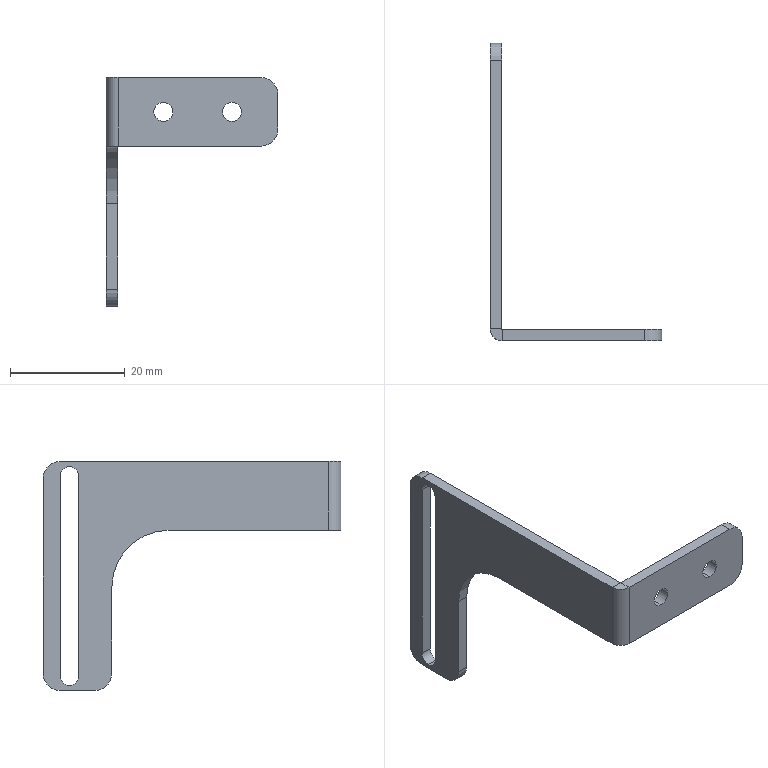Part | SolidWorks | features Fillet 2, ICE 2, FlatPattern 1, HoleWzd 1, SMBaseFlange 1, SheetMetal 1 | 1 solid | 29 faces | box 30 x 52 x 40 mm | volume 2330 mm3 | cylinder 15 | plane 14 | commonest cylinder face diameters 6 x5 3.3 x4 3.2 x3 0.2 x1 4.2 x1 20 x1
STEP:
#1=CARTESIAN_POINT('',(8.,-2.,32.35));
#2=VERTEX_POINT('',#1);
#3=CARTESIAN_POINT('',(8.,-2.,35.65));
#4=VERTEX_POINT('',#3);
#5=CARTESIAN_POINT('',(8.,-2.,34.));
#6=DIRECTION('',(0.,1.,0.));
#7=DIRECTION('',(0.,0.,1.));
#8=AXIS2_PLACEMENT_3D('',#5,#6,#7);
#9=CIRCLE('',#8,1.65);
#10=EDGE_CURVE('',#2,#4,#9,.T.);
#11=ORIENTED_EDGE('',*,*,#10,.F.);
#12=CARTESIAN_POINT('',(8.,0.,32.35));
#13=VERTEX_POINT('',#12);
#14=CARTESIAN_POINT('',(8.,0.,32.35));
#15=DIRECTION('',(0.,1.,0.));
#16=VECTOR('',#15,1000.);
#17=LINE('',#14,#16);
#18=EDGE_CURVE('',#2,#13,#17,.T.);
#19=ORIENTED_EDGE('',*,*,#18,.T.);
#20=CARTESIAN_POINT('',(8.,0.,35.65));
#21=VERTEX_POINT('',#20);
#22=CARTESIAN_POINT('',(8.,0.,34.));
#23=DIRECTION('',(0.,1.,0.));
#24=DIRECTION('',(0.,0.,1.));
#25=AXIS2_PLACEMENT_3D('',#22,#23,#24);
#26=CIRCLE('',#25,1.65);
#27=EDGE_CURVE('',#13,#21,#26,.T.);
#28=ORIENTED_EDGE('',*,*,#27,.T.);
#29=CARTESIAN_POINT('',(8.,0.,35.65));
#30=DIRECTION('',(0.,1.,0.));
#31=VECTOR('',#30,1000.);
#32=LINE('',#29,#31);
#33=EDGE_CURVE('',#4,#21,#32,.T.);
#34=ORIENTED_EDGE('',*,*,#33,.F.);
#35=EDGE_LOOP('',(#11,#19,#28,#34));
#36=FACE_OUTER_BOUND('',#35,.T.);
#37=CARTESIAN_POINT('',(8.,0.,34.));
#38=DIRECTION('',(0.,1.,0.));
#39=DIRECTION('',(0.,0.,1.));
#40=AXIS2_PLACEMENT_3D('',#37,#38,#39);
#41=CYLINDRICAL_SURFACE('',#40,1.65);
#42=ADVANCED_FACE('',(#36),#41,.F.);
#43=CARTESIAN_POINT('',(20.,-2.,32.35));
#44=VERTEX_POINT('',#43);
#45=CARTESIAN_POINT('',(20.,-2.,35.65));
#46=VERTEX_POINT('',#45);
#47=CARTESIAN_POINT('',(20.,-2.,34.));
#48=DIRECTION('',(0.,1.,0.));
#49=DIRECTION('',(0.,0.,1.));
#50=AXIS2_PLACEMENT_3D('',#47,#48,#49);
#51=CIRCLE('',#50,1.65);
#52=EDGE_CURVE('',#44,#46,#51,.T.);
#53=ORIENTED_EDGE('',*,*,#52,.F.);
#54=CARTESIAN_POINT('',(20.,0.,32.35));
#55=VERTEX_POINT('',#54);
#56=CARTESIAN_POINT('',(20.,0.,32.35));
#57=DIRECTION('',(0.,1.,0.));
#58=VECTOR('',#57,1000.);
#59=LINE('',#56,#58);
#60=EDGE_CURVE('',#44,#55,#59,.T.);
#61=ORIENTED_EDGE('',*,*,#60,.T.);
#62=CARTESIAN_POINT('',(20.,0.,35.65));
#63=VERTEX_POINT('',#62);
#64=CARTESIAN_POINT('',(20.,0.,34.));
#65=DIRECTION('',(0.,1.,0.));
#66=DIRECTION('',(0.,0.,1.));
#67=AXIS2_PLACEMENT_3D('',#64,#65,#66);
#68=CIRCLE('',#67,1.65);
#69=EDGE_CURVE('',#55,#63,#68,.T.);
#70=ORIENTED_EDGE('',*,*,#69,.T.);
#71=CARTESIAN_POINT('',(20.,0.,35.65));
#72=DIRECTION('',(0.,1.,0.));
#73=VECTOR('',#72,1000.);
#74=LINE('',#71,#73);
#75=EDGE_CURVE('',#46,#63,#74,.T.);
#76=ORIENTED_EDGE('',*,*,#75,.F.);
#77=EDGE_LOOP('',(#53,#61,#70,#76));
#78=FACE_OUTER_BOUND('',#77,.T.);
#79=CARTESIAN_POINT('',(20.,0.,34.));
#80=DIRECTION('',(0.,1.,0.));
#81=DIRECTION('',(0.,0.,1.));
#82=AXIS2_PLACEMENT_3D('',#79,#80,#81);
#83=CYLINDRICAL_SURFACE('',#82,1.65);
#84=ADVANCED_FACE('',(#78),#83,.F.);
#85=CARTESIAN_POINT('',(-2.,45.4,0.9));
#86=VERTEX_POINT('',#85);
#87=CARTESIAN_POINT('',(-2.,47.,2.5));
#88=VERTEX_POINT('',#87);
#89=CARTESIAN_POINT('',(-2.,45.4,2.5));
#90=DIRECTION('',(1.,0.,0.));
#91=DIRECTION('',(0.,0.,-1.));
#92=AXIS2_PLACEMENT_3D('',#89,#90,#91);
#93=CIRCLE('',#92,1.6);
#94=EDGE_CURVE('',#86,#88,#93,.T.);
#95=ORIENTED_EDGE('',*,*,#94,.F.);
#96=CARTESIAN_POINT('',(0.,45.4,0.9));
#97=VERTEX_POINT('',#96);
#98=CARTESIAN_POINT('',(-2.,45.4,0.9));
#99=DIRECTION('',(1.,0.,0.));
#100=VECTOR('',#99,1000.);
#101=LINE('',#98,#100);
#102=EDGE_CURVE('',#86,#97,#101,.T.);
#103=ORIENTED_EDGE('',*,*,#102,.T.);
#104=CARTESIAN_POINT('',(0.,47.,2.5));
#105=VERTEX_POINT('',#104);
#106=CARTESIAN_POINT('',(0.,45.4,2.5));
#107=DIRECTION('',(1.,0.,0.));
#108=DIRECTION('',(0.,0.,-1.));
#109=AXIS2_PLACEMENT_3D('',#106,#107,#108);
#110=CIRCLE('',#109,1.6);
#111=EDGE_CURVE('',#97,#105,#110,.T.);
#112=ORIENTED_EDGE('',*,*,#111,.T.);
#113=CARTESIAN_POINT('',(-2.,47.,2.5));
#114=DIRECTION('',(1.,0.,0.));
#115=VECTOR('',#114,1000.);
#116=LINE('',#113,#115);
#117=EDGE_CURVE('',#88,#105,#116,.T.);
#118=ORIENTED_EDGE('',*,*,#117,.F.);
#119=EDGE_LOOP('',(#95,#103,#112,#118));
#120=FACE_OUTER_BOUND('',#119,.T.);
#121=CARTESIAN_POINT('',(-2.,45.4,2.5));
#122=DIRECTION('',(1.,0.,0.));
#123=DIRECTION('',(0.,0.,-1.));
#124=AXIS2_PLACEMENT_3D('',#121,#122,#123);
#125=CYLINDRICAL_SURFACE('',#124,1.6);
#126=ADVANCED_FACE('',(#120),#125,.F.);
#127=CARTESIAN_POINT('',(-2.,41.,0.));
#128=VERTEX_POINT('',#127);
#129=CARTESIAN_POINT('',(0.,41.,0.));
#130=VERTEX_POINT('',#129);
#131=CARTESIAN_POINT('',(-2.,41.,0.));
#132=DIRECTION('',(1.,0.,0.));
#133=VECTOR('',#132,1000.);
#134=LINE('',#131,#133);
#135=EDGE_CURVE('',#128,#130,#134,.T.);
#136=ORIENTED_EDGE('',*,*,#135,.F.);
#137=CARTESIAN_POINT('',(-2.,47.,0.));
#138=VERTEX_POINT('',#137);
#139=CARTESIAN_POINT('',(-2.,0.,0.));
#140=DIRECTION('',(0.,-1.,0.));
#141=VECTOR('',#140,1000.);
#142=LINE('',#139,#141);
#143=EDGE_CURVE('',#138,#128,#142,.T.);
#144=ORIENTED_EDGE('',*,*,#143,.F.);
#145=CARTESIAN_POINT('',(0.,47.,0.));
#146=VERTEX_POINT('',#145);
#147=CARTESIAN_POINT('',(-2.,47.,0.));
#148=DIRECTION('',(1.,0.,0.));
#149=VECTOR('',#148,1000.);
#150=LINE('',#147,#149);
#151=EDGE_CURVE('',#138,#146,#150,.T.);
#152=ORIENTED_EDGE('',*,*,#151,.T.);
#153=CARTESIAN_POINT('',(0.,0.,0.));
#154=DIRECTION('',(0.,-1.,0.));
#155=VECTOR('',#154,1000.);
#156=LINE('',#153,#155);
#157=EDGE_CURVE('',#146,#130,#156,.T.);
#158=ORIENTED_EDGE('',*,*,#157,.T.);
#159=EDGE_LOOP('',(#136,#144,#152,#158));
#160=FACE_OUTER_BOUND('',#159,.T.);
#161=CARTESIAN_POINT('',(0.1,-2.,0.));
#162=DIRECTION('',(0.,0.,-1.));
#163=DIRECTION('',(-1.,0.,0.));
#164=AXIS2_PLACEMENT_3D('',#161,#162,#163);
#165=PLANE('',#164);
#166=ADVANCED_FACE('',(#160),#165,.T.);
#167=CARTESIAN_POINT('',(0.,43.8,37.5));
#168=VERTEX_POINT('',#167);
#169=CARTESIAN_POINT('',(0.,43.8,2.5));
#170=VERTEX_POINT('',#169);
#171=CARTESIAN_POINT('',(0.,43.8,0.));
#172=DIRECTION('',(0.,0.,-1.));
#173=VECTOR('',#172,1000.);
#174=LINE('',#171,#173);
#175=EDGE_CURVE('',#168,#170,#174,.T.);
#176=ORIENTED_EDGE('',*,*,#175,.F.);
#177=CARTESIAN_POINT('',(0.,47.,37.5));
#178=VERTEX_POINT('',#177);
#179=CARTESIAN_POINT('',(0.,45.4,37.5));
#180=DIRECTION('',(1.,0.,0.));
#181=DIRECTION('',(0.,0.,-1.));
#182=AXIS2_PLACEMENT_3D('',#179,#180,#181);
#183=CIRCLE('',#182,1.6);
#184=EDGE_CURVE('',#178,#168,#183,.T.);
#185=ORIENTED_EDGE('',*,*,#184,.F.);
#186=CARTESIAN_POINT('',(0.,47.,0.));
#187=DIRECTION('',(0.,0.,-1.));
#188=VECTOR('',#187,1000.);
#189=LINE('',#186,#188);
#190=EDGE_CURVE('',#178,#105,#189,.T.);
#191=ORIENTED_EDGE('',*,*,#190,.T.);
#192=ORIENTED_EDGE('',*,*,#111,.F.);
#193=CARTESIAN_POINT('',(0.,45.4,2.5));
#194=DIRECTION('',(1.,0.,0.));
#195=DIRECTION('',(0.,0.,-1.));
#196=AXIS2_PLACEMENT_3D('',#193,#194,#195);
#197=CIRCLE('',#196,1.6);
#198=EDGE_CURVE('',#170,#97,#197,.T.);
#199=ORIENTED_EDGE('',*,*,#198,.F.);
#200=EDGE_LOOP('',(#176,#185,#191,#192,#199));
#201=FACE_BOUND('',#200,.T.);
#202=CARTESIAN_POINT('',(0.,50.,37.));
#203=VERTEX_POINT('',#202);
#204=CARTESIAN_POINT('',(0.,50.,3.));
#205=VERTEX_POINT('',#204);
#206=CARTESIAN_POINT('',(0.,50.,40.));
#207=DIRECTION('',(0.,0.,-1.));
#208=VECTOR('',#207,1000.);
#209=LINE('',#206,#208);
#210=EDGE_CURVE('',#203,#205,#209,.T.);
#211=ORIENTED_EDGE('',*,*,#210,.F.);
#212=CARTESIAN_POINT('',(0.,47.,40.));
#213=VERTEX_POINT('',#212);
#214=CARTESIAN_POINT('',(0.,47.,37.));
#215=DIRECTION('',(1.,0.,0.));
#216=DIRECTION('',(0.,0.,-1.));
#217=AXIS2_PLACEMENT_3D('',#214,#215,#216);
#218=CIRCLE('',#217,3.);
#219=EDGE_CURVE('',#203,#213,#218,.T.);
#220=ORIENTED_EDGE('',*,*,#219,.T.);
#221=CARTESIAN_POINT('',(0.,0.1,40.));
#222=VERTEX_POINT('',#221);
#223=CARTESIAN_POINT('',(0.,0.,40.));
#224=DIRECTION('',(0.,-1.,0.));
#225=VECTOR('',#224,1000.);
#226=LINE('',#223,#225);
#227=EDGE_CURVE('',#213,#222,#226,.T.);
#228=ORIENTED_EDGE('',*,*,#227,.T.);
#229=CARTESIAN_POINT('',(0.,0.1,28.));
#230=VERTEX_POINT('',#229);
#231=CARTESIAN_POINT('',(0.,0.1,40.));
#232=DIRECTION('',(0.,0.,-1.));
#233=VECTOR('',#232,1000.);
#234=LINE('',#231,#233);
#235=EDGE_CURVE('',#222,#230,#234,.T.);
#236=ORIENTED_EDGE('',*,*,#235,.T.);
#237=CARTESIAN_POINT('',(0.,28.,28.));
#238=VERTEX_POINT('',#237);
#239=CARTESIAN_POINT('',(0.,0.,28.));
#240=DIRECTION('',(0.,1.,0.));
#241=VECTOR('',#240,1000.);
#242=LINE('',#239,#241);
#243=EDGE_CURVE('',#230,#238,#242,.T.);
#244=ORIENTED_EDGE('',*,*,#243,.T.);
#245=CARTESIAN_POINT('',(0.,38.,18.));
#246=VERTEX_POINT('',#245);
#247=CARTESIAN_POINT('',(0.,28.,18.));
#248=DIRECTION('',(-1.,0.,0.));
#249=DIRECTION('',(0.,0.,-1.));
#250=AXIS2_PLACEMENT_3D('',#247,#248,#249);
#251=CIRCLE('',#250,10.);
#252=EDGE_CURVE('',#238,#246,#251,.T.);
#253=ORIENTED_EDGE('',*,*,#252,.T.);
#254=CARTESIAN_POINT('',(0.,38.,3.));
#255=VERTEX_POINT('',#254);
#256=CARTESIAN_POINT('',(0.,38.,0.));
#257=DIRECTION('',(0.,0.,-1.));
#258=VECTOR('',#257,1000.);
#259=LINE('',#256,#258);
#260=EDGE_CURVE('',#246,#255,#259,.T.);
#261=ORIENTED_EDGE('',*,*,#260,.T.);
#262=CARTESIAN_POINT('',(0.,41.,3.));
#263=DIRECTION('',(1.,0.,0.));
#264=DIRECTION('',(0.,0.,-1.));
#265=AXIS2_PLACEMENT_3D('',#262,#263,#264);
#266=CIRCLE('',#265,3.);
#267=EDGE_CURVE('',#255,#130,#266,.T.);
#268=ORIENTED_EDGE('',*,*,#267,.T.);
#269=ORIENTED_EDGE('',*,*,#157,.F.);
#270=CARTESIAN_POINT('',(0.,47.,3.));
#271=DIRECTION('',(1.,0.,0.));
#272=DIRECTION('',(0.,0.,-1.));
#273=AXIS2_PLACEMENT_3D('',#270,#271,#272);
#274=CIRCLE('',#273,3.);
#275=EDGE_CURVE('',#146,#205,#274,.T.);
#276=ORIENTED_EDGE('',*,*,#275,.T.);
#277=EDGE_LOOP('',(#211,#220,#228,#236,#244,#253,#261,#268,#269,#276));
#278=FACE_OUTER_BOUND('',#277,.T.);
#279=CARTESIAN_POINT('',(0.,0.,40.));
#280=DIRECTION('',(1.,0.,0.));
#281=DIRECTION('',(0.,0.,-1.));
#282=AXIS2_PLACEMENT_3D('',#279,#280,#281);
#283=PLANE('',#282);
#284=ADVANCED_FACE('',(#201,#278),#283,.T.);
#285=CARTESIAN_POINT('',(-2.,47.,37.5));
#286=VERTEX_POINT('',#285);
#287=CARTESIAN_POINT('',(-2.,43.8,37.5));
#288=VERTEX_POINT('',#287);
#289=CARTESIAN_POINT('',(-2.,45.4,37.5));
#290=DIRECTION('',(1.,0.,0.));
#291=DIRECTION('',(0.,0.,-1.));
#292=AXIS2_PLACEMENT_3D('',#289,#290,#291);
#293=CIRCLE('',#292,1.6);
#294=EDGE_CURVE('',#286,#288,#293,.T.);
#295=ORIENTED_EDGE('',*,*,#294,.T.);
#296=CARTESIAN_POINT('',(-2.,43.8,2.5));
#297=VERTEX_POINT('',#296);
#298=CARTESIAN_POINT('',(-2.,43.8,0.));
#299=DIRECTION('',(0.,0.,-1.));
#300=VECTOR('',#299,1000.);
#301=LINE('',#298,#300);
#302=EDGE_CURVE('',#288,#297,#301,.T.);
#303=ORIENTED_EDGE('',*,*,#302,.T.);
#304=CARTESIAN_POINT('',(-2.,45.4,2.5));
#305=DIRECTION('',(1.,0.,0.));
#306=DIRECTION('',(0.,0.,-1.));
#307=AXIS2_PLACEMENT_3D('',#304,#305,#306);
#308=CIRCLE('',#307,1.6);
#309=EDGE_CURVE('',#297,#86,#308,.T.);
#310=ORIENTED_EDGE('',*,*,#309,.T.);
#311=ORIENTED_EDGE('',*,*,#94,.T.);
#312=CARTESIAN_POINT('',(-2.,47.,0.));
#313=DIRECTION('',(0.,0.,-1.));
#314=VECTOR('',#313,1000.);
#315=LINE('',#312,#314);
#316=EDGE_CURVE('',#286,#88,#315,.T.);
#317=ORIENTED_EDGE('',*,*,#316,.F.);
#318=EDGE_LOOP('',(#295,#303,#310,#311,#317));
#319=FACE_BOUND('',#318,.T.);
#320=CARTESIAN_POINT('',(-2.,47.,40.));
#321=VERTEX_POINT('',#320);
#322=CARTESIAN_POINT('',(-2.,0.1,40.));
#323=VERTEX_POINT('',#322);
#324=CARTESIAN_POINT('',(-2.,0.,40.));
#325=DIRECTION('',(0.,-1.,0.));
#326=VECTOR('',#325,1000.);
#327=LINE('',#324,#326);
#328=EDGE_CURVE('',#321,#323,#327,.T.);
#329=ORIENTED_EDGE('',*,*,#328,.F.);
#330=CARTESIAN_POINT('',(-2.,50.,37.));
#331=VERTEX_POINT('',#330);
#332=CARTESIAN_POINT('',(-2.,47.,37.));
#333=DIRECTION('',(-1.,0.,0.));
#334=DIRECTION('',(0.,0.,-1.));
#335=AXIS2_PLACEMENT_3D('',#332,#333,#334);
#336=CIRCLE('',#335,3.);
#337=EDGE_CURVE('',#321,#331,#336,.T.);
#338=ORIENTED_EDGE('',*,*,#337,.T.);
#339=CARTESIAN_POINT('',(-2.,50.,3.));
#340=VERTEX_POINT('',#339);
#341=CARTESIAN_POINT('',(-2.,50.,40.));
#342=DIRECTION('',(0.,0.,-1.));
#343=VECTOR('',#342,1000.);
#344=LINE('',#341,#343);
#345=EDGE_CURVE('',#331,#340,#344,.T.);
#346=ORIENTED_EDGE('',*,*,#345,.T.);
#347=CARTESIAN_POINT('',(-2.,47.,3.));
#348=DIRECTION('',(1.,0.,0.));
#349=DIRECTION('',(0.,0.,-1.));
#350=AXIS2_PLACEMENT_3D('',#347,#348,#349);
#351=CIRCLE('',#350,3.);
#352=EDGE_CURVE('',#138,#340,#351,.T.);
#353=ORIENTED_EDGE('',*,*,#352,.F.);
#354=ORIENTED_EDGE('',*,*,#143,.T.);
#355=CARTESIAN_POINT('',(-2.,38.,3.));
#356=VERTEX_POINT('',#355);
#357=CARTESIAN_POINT('',(-2.,41.,3.));
#358=DIRECTION('',(1.,0.,0.));
#359=DIRECTION('',(0.,0.,-1.));
#360=AXIS2_PLACEMENT_3D('',#357,#358,#359);
#361=CIRCLE('',#360,3.);
#362=EDGE_CURVE('',#356,#128,#361,.T.);
#363=ORIENTED_EDGE('',*,*,#362,.F.);
#364=CARTESIAN_POINT('',(-2.,38.,18.));
#365=VERTEX_POINT('',#364);
#366=CARTESIAN_POINT('',(-2.,38.,0.));
#367=DIRECTION('',(0.,0.,-1.));
#368=VECTOR('',#367,1000.);
#369=LINE('',#366,#368);
#370=EDGE_CURVE('',#365,#356,#369,.T.);
#371=ORIENTED_EDGE('',*,*,#370,.F.);
#372=CARTESIAN_POINT('',(-2.,28.,28.));
#373=VERTEX_POINT('',#372);
#374=CARTESIAN_POINT('',(-2.,28.,18.));
#375=DIRECTION('',(-1.,0.,0.));
#376=DIRECTION('',(0.,0.,-1.));
#377=AXIS2_PLACEMENT_3D('',#374,#375,#376);
#378=CIRCLE('',#377,10.);
#379=EDGE_CURVE('',#373,#365,#378,.T.);
#380=ORIENTED_EDGE('',*,*,#379,.F.);
#381=CARTESIAN_POINT('',(-2.,0.1,28.));
#382=VERTEX_POINT('',#381);
#383=CARTESIAN_POINT('',(-2.,0.,28.));
#384=DIRECTION('',(0.,1.,0.));
#385=VECTOR('',#384,1000.);
#386=LINE('',#383,#385);
#387=EDGE_CURVE('',#382,#373,#386,.T.);
#388=ORIENTED_EDGE('',*,*,#387,.F.);
#389=CARTESIAN_POINT('',(-2.,0.1,40.));
#390=DIRECTION('',(0.,0.,-1.));
#391=VECTOR('',#390,1000.);
#392=LINE('',#389,#391);
#393=EDGE_CURVE('',#323,#382,#392,.T.);
#394=ORIENTED_EDGE('',*,*,#393,.F.);
#395=EDGE_LOOP('',(#329,#338,#346,#353,#354,#363,#371,#380,#388,#394));
#396=FACE_OUTER_BOUND('',#395,.T.);
#397=CARTESIAN_POINT('',(-2.,0.,40.));
#398=DIRECTION('',(1.,0.,0.));
#399=DIRECTION('',(0.,0.,-1.));
#400=AXIS2_PLACEMENT_3D('',#397,#398,#399);
#401=PLANE('',#400);
#402=ADVANCED_FACE('',(#319,#396),#401,.F.);
#403=CARTESIAN_POINT('',(0.1,0.,40.));
#404=VERTEX_POINT('',#403);
#405=CARTESIAN_POINT('',(0.1,-2.,40.));
#406=VERTEX_POINT('',#405);
#407=CARTESIAN_POINT('',(0.1,0.,40.));
#408=DIRECTION('',(0.,-1.,0.));
#409=VECTOR('',#408,1000.);
#410=LINE('',#407,#409);
#411=EDGE_CURVE('',#404,#406,#410,.T.);
#412=ORIENTED_EDGE('',*,*,#411,.F.);
#413=CARTESIAN_POINT('',(0.1,0.1,40.));
#414=DIRECTION('',(0.,0.,1.));
#415=DIRECTION('',(-1.,0.,0.));
#416=AXIS2_PLACEMENT_3D('',#413,#414,#415);
#417=CIRCLE('',#416,0.1);
#418=EDGE_CURVE('',#222,#404,#417,.T.);
#419=ORIENTED_EDGE('',*,*,#418,.F.);
#420=CARTESIAN_POINT('',(-2.,0.1,40.));
#421=DIRECTION('',(1.,0.,0.));
#422=VECTOR('',#421,1000.);
#423=LINE('',#420,#422);
#424=EDGE_CURVE('',#323,#222,#423,.T.);
#425=ORIENTED_EDGE('',*,*,#424,.F.);
#426=CARTESIAN_POINT('',(0.1,0.1,40.));
#427=DIRECTION('',(0.,0.,1.));
#428=DIRECTION('',(1.,0.,0.));
#429=AXIS2_PLACEMENT_3D('',#426,#427,#428);
#430=CIRCLE('',#429,2.1);
#431=EDGE_CURVE('',#323,#406,#430,.T.);
#432=ORIENTED_EDGE('',*,*,#431,.T.);
#433=EDGE_LOOP('',(#412,#419,#425,#432));
#434=FACE_OUTER_BOUND('',#433,.T.);
#435=CARTESIAN_POINT('',(0.1,0.,40.));
#436=DIRECTION('',(0.,0.,1.));
#437=DIRECTION('',(1.,0.,0.));
#438=AXIS2_PLACEMENT_3D('',#435,#436,#437);
#439=PLANE('',#438);
#440=ADVANCED_FACE('',(#434),#439,.T.);
#441=CARTESIAN_POINT('',(25.,-2.,40.));
#442=VERTEX_POINT('',#441);
#443=CARTESIAN_POINT('',(0.,-2.,40.));
#444=DIRECTION('',(1.,0.,0.));
#445=VECTOR('',#444,1000.);
#446=LINE('',#443,#445);
#447=EDGE_CURVE('',#406,#442,#446,.T.);
#448=ORIENTED_EDGE('',*,*,#447,.T.);
#449=CARTESIAN_POINT('',(25.,0.,40.));
#450=VERTEX_POINT('',#449);
#451=CARTESIAN_POINT('',(25.,0.1,40.));
#452=DIRECTION('',(0.,1.,0.));
#453=VECTOR('',#452,1000.);
#454=LINE('',#451,#453);
#455=EDGE_CURVE('',#442,#450,#454,.T.);
#456=ORIENTED_EDGE('',*,*,#455,.T.);
#457=CARTESIAN_POINT('',(0.,0.,40.));
#458=DIRECTION('',(1.,0.,0.));
#459=VECTOR('',#458,1000.);
#460=LINE('',#457,#459);
#461=EDGE_CURVE('',#404,#450,#460,.T.);
#462=ORIENTED_EDGE('',*,*,#461,.F.);
#463=ORIENTED_EDGE('',*,*,#411,.T.);
#464=EDGE_LOOP('',(#448,#456,#462,#463));
#465=FACE_OUTER_BOUND('',#464,.T.);
#466=CARTESIAN_POINT('',(-2.,0.1,40.));
#467=DIRECTION('',(0.,0.,1.));
#468=DIRECTION('',(1.,0.,0.));
#469=AXIS2_PLACEMENT_3D('',#466,#467,#468);
#470=PLANE('',#469);
#471=ADVANCED_FACE('',(#465),#470,.T.);
#472=CARTESIAN_POINT('',(8.,-2.,34.));
#473=DIRECTION('',(0.,1.,0.));
#474=DIRECTION('',(0.,0.,1.));
#475=AXIS2_PLACEMENT_3D('',#472,#473,#474);
#476=CIRCLE('',#475,1.65);
#477=EDGE_CURVE('',#4,#2,#476,.T.);
#478=ORIENTED_EDGE('',*,*,#477,.T.);
#479=ORIENTED_EDGE('',*,*,#10,.T.);
#480=EDGE_LOOP('',(#478,#479));
#481=FACE_BOUND('',#480,.T.);
#482=CARTESIAN_POINT('',(20.,-2.,34.));
#483=DIRECTION('',(0.,1.,0.));
#484=DIRECTION('',(0.,0.,1.));
#485=AXIS2_PLACEMENT_3D('',#482,#483,#484);
#486=CIRCLE('',#485,1.65);
#487=EDGE_CURVE('',#46,#44,#486,.T.);
#488=ORIENTED_EDGE('',*,*,#487,.T.);
#489=ORIENTED_EDGE('',*,*,#52,.T.);
#490=EDGE_LOOP('',(#488,#489));
#491=FACE_BOUND('',#490,.T.);
#492=CARTESIAN_POINT('',(0.1,-2.,28.));
#493=VERTEX_POINT('',#492);
#494=CARTESIAN_POINT('',(25.,-2.,28.));
#495=VERTEX_POINT('',#494);
#496=CARTESIAN_POINT('',(-2.,-2.,28.));
#497=DIRECTION('',(1.,0.,0.));
#498=VECTOR('',#497,1000.);
#499=LINE('',#496,#498);
#500=EDGE_CURVE('',#493,#495,#499,.T.);
#501=ORIENTED_EDGE('',*,*,#500,.T.);
#502=CARTESIAN_POINT('',(28.,-2.,31.));
#503=VERTEX_POINT('',#502);
#504=CARTESIAN_POINT('',(25.,-2.,31.));
#505=DIRECTION('',(0.,-1.,0.));
#506=DIRECTION('',(0.,0.,1.));
#507=AXIS2_PLACEMENT_3D('',#504,#505,#506);
#508=CIRCLE('',#507,3.);
#509=EDGE_CURVE('',#495,#503,#508,.T.);
#510=ORIENTED_EDGE('',*,*,#509,.T.);
#511=CARTESIAN_POINT('',(28.,-2.,37.));
#512=VERTEX_POINT('',#511);
#513=CARTESIAN_POINT('',(28.,-2.,40.));
#514=DIRECTION('',(0.,0.,-1.));
#515=VECTOR('',#514,1000.);
#516=LINE('',#513,#515);
#517=EDGE_CURVE('',#512,#503,#516,.T.);
#518=ORIENTED_EDGE('',*,*,#517,.F.);
#519=CARTESIAN_POINT('',(25.,-2.,37.));
#520=DIRECTION('',(0.,-1.,0.));
#521=DIRECTION('',(0.,0.,1.));
#522=AXIS2_PLACEMENT_3D('',#519,#520,#521);
#523=CIRCLE('',#522,3.);
#524=EDGE_CURVE('',#512,#442,#523,.T.);
#525=ORIENTED_EDGE('',*,*,#524,.T.);
#526=ORIENTED_EDGE('',*,*,#447,.F.);
#527=CARTESIAN_POINT('',(0.1,-2.,40.));
#528=DIRECTION('',(0.,0.,-1.));
#529=VECTOR('',#528,1000.);
#530=LINE('',#527,#529);
#531=EDGE_CURVE('',#406,#493,#530,.T.);
#532=ORIENTED_EDGE('',*,*,#531,.T.);
#533=EDGE_LOOP('',(#501,#510,#518,#525,#526,#532));
#534=FACE_OUTER_BOUND('',#533,.T.);
#535=CARTESIAN_POINT('',(0.,-2.,40.));
#536=DIRECTION('',(0.,1.,0.));
#537=DIRECTION('',(0.,0.,1.));
#538=AXIS2_PLACEMENT_3D('',#535,#536,#537);
#539=PLANE('',#538);
#540=ADVANCED_FACE('',(#481,#491,#534),#539,.F.);
#541=ORIENTED_EDGE('',*,*,#517,.T.);
#542=CARTESIAN_POINT('',(28.,0.,31.));
#543=VERTEX_POINT('',#542);
#544=CARTESIAN_POINT('',(28.,0.,31.));
#545=DIRECTION('',(0.,1.,0.));
#546=VECTOR('',#545,1000.);
#547=LINE('',#544,#546);
#548=EDGE_CURVE('',#503,#543,#547,.T.);
#549=ORIENTED_EDGE('',*,*,#548,.T.);
#550=CARTESIAN_POINT('',(28.,0.,37.));
#551=VERTEX_POINT('',#550);
#552=CARTESIAN_POINT('',(28.,0.,40.));
#553=DIRECTION('',(0.,0.,-1.));
#554=VECTOR('',#553,1000.);
#555=LINE('',#552,#554);
#556=EDGE_CURVE('',#551,#543,#555,.T.);
#557=ORIENTED_EDGE('',*,*,#556,.F.);
#558=CARTESIAN_POINT('',(28.,0.,37.));
#559=DIRECTION('',(0.,-1.,0.));
#560=VECTOR('',#559,1000.);
#561=LINE('',#558,#560);
#562=EDGE_CURVE('',#551,#512,#561,.T.);
#563=ORIENTED_EDGE('',*,*,#562,.T.);
#564=EDGE_LOOP('',(#541,#549,#557,#563));
#565=FACE_OUTER_BOUND('',#564,.T.);
#566=CARTESIAN_POINT('',(28.,0.,40.));
#567=DIRECTION('',(1.,0.,0.));
#568=DIRECTION('',(0.,0.,-1.));
#569=AXIS2_PLACEMENT_3D('',#566,#567,#568);
#570=PLANE('',#569);
#571=ADVANCED_FACE('',(#565),#570,.T.);
#572=CARTESIAN_POINT('',(8.,0.,34.));
#573=DIRECTION('',(0.,1.,0.));
#574=DIRECTION('',(0.,0.,1.));
#575=AXIS2_PLACEMENT_3D('',#572,#573,#574);
#576=CIRCLE('',#575,1.65);
#577=EDGE_CURVE('',#21,#13,#576,.T.);
#578=ORIENTED_EDGE('',*,*,#577,.F.);
#579=ORIENTED_EDGE('',*,*,#27,.F.);
#580=EDGE_LOOP('',(#578,#579));
#581=FACE_BOUND('',#580,.T.);
#582=CARTESIAN_POINT('',(20.,0.,34.));
#583=DIRECTION('',(0.,1.,0.));
#584=DIRECTION('',(0.,0.,1.));
#585=AXIS2_PLACEMENT_3D('',#582,#583,#584);
#586=CIRCLE('',#585,1.65);
#587=EDGE_CURVE('',#63,#55,#586,.T.);
#588=ORIENTED_EDGE('',*,*,#587,.F.);
#589=ORIENTED_EDGE('',*,*,#69,.F.);
#590=EDGE_LOOP('',(#588,#589));
#591=FACE_BOUND('',#590,.T.);
#592=ORIENTED_EDGE('',*,*,#556,.T.);
#593=CARTESIAN_POINT('',(25.,0.,28.));
#594=VERTEX_POINT('',#593);
#595=CARTESIAN_POINT('',(25.,0.,31.));
#596=DIRECTION('',(0.,1.,0.));
#597=DIRECTION('',(0.,0.,1.));
#598=AXIS2_PLACEMENT_3D('',#595,#596,#597);
#599=CIRCLE('',#598,3.);
#600=EDGE_CURVE('',#543,#594,#599,.T.);
#601=ORIENTED_EDGE('',*,*,#600,.T.);
#602=CARTESIAN_POINT('',(0.1,0.,28.));
#603=VERTEX_POINT('',#602);
#604=CARTESIAN_POINT('',(0.,0.,28.));
#605=DIRECTION('',(1.,0.,0.));
#606=VECTOR('',#605,1000.);
#607=LINE('',#604,#606);
#608=EDGE_CURVE('',#603,#594,#607,.T.);
#609=ORIENTED_EDGE('',*,*,#608,.F.);
#610=CARTESIAN_POINT('',(0.1,0.,40.));
#611=DIRECTION('',(0.,0.,-1.));
#612=VECTOR('',#611,1000.);
#613=LINE('',#610,#612);
#614=EDGE_CURVE('',#404,#603,#613,.T.);
#615=ORIENTED_EDGE('',*,*,#614,.F.);
#616=ORIENTED_EDGE('',*,*,#461,.T.);
#617=CARTESIAN_POINT('',(25.,0.,37.));
#618=DIRECTION('',(0.,1.,0.));
#619=DIRECTION('',(0.,0.,1.));
#620=AXIS2_PLACEMENT_3D('',#617,#618,#619);
#621=CIRCLE('',#620,3.);
#622=EDGE_CURVE('',#450,#551,#621,.T.);
#623=ORIENTED_EDGE('',*,*,#622,.T.);
#624=EDGE_LOOP('',(#592,#601,#609,#615,#616,#623));
#625=FACE_OUTER_BOUND('',#624,.T.);
#626=CARTESIAN_POINT('',(0.,0.,40.));
#627=DIRECTION('',(0.,1.,0.));
#628=DIRECTION('',(0.,0.,1.));
#629=AXIS2_PLACEMENT_3D('',#626,#627,#628);
#630=PLANE('',#629);
#631=ADVANCED_FACE('',(#581,#591,#625),#630,.T.);
#632=CARTESIAN_POINT('',(0.1,0.1,28.));
#633=DIRECTION('',(0.,0.,1.));
#634=DIRECTION('',(1.,0.,0.));
#635=AXIS2_PLACEMENT_3D('',#632,#633,#634);
#636=CIRCLE('',#635,0.1);
#637=EDGE_CURVE('',#230,#603,#636,.T.);
#638=ORIENTED_EDGE('',*,*,#637,.F.);
#639=ORIENTED_EDGE('',*,*,#235,.F.);
#640=ORIENTED_EDGE('',*,*,#418,.T.);
#641=ORIENTED_EDGE('',*,*,#614,.T.);
#642=EDGE_LOOP('',(#638,#639,#640,#641));
#643=FACE_OUTER_BOUND('',#642,.T.);
#644=CARTESIAN_POINT('',(0.1,0.1,40.));
#645=DIRECTION('',(0.,0.,-1.));
#646=DIRECTION('',(-1.,0.,0.));
#647=AXIS2_PLACEMENT_3D('',#644,#645,#646);
#648=CYLINDRICAL_SURFACE('',#647,0.1);
#649=ADVANCED_FACE('',(#643),#648,.F.);
#650=ORIENTED_EDGE('',*,*,#345,.F.);
#651=CARTESIAN_POINT('',(0.,50.,37.));
#652=DIRECTION('',(1.,0.,0.));
#653=VECTOR('',#652,1000.);
#654=LINE('',#651,#653);
#655=EDGE_CURVE('',#331,#203,#654,.T.);
#656=ORIENTED_EDGE('',*,*,#655,.T.);
#657=ORIENTED_EDGE('',*,*,#210,.T.);
#658=CARTESIAN_POINT('',(-2.,50.,3.));
#659=DIRECTION('',(1.,0.,0.));
#660=VECTOR('',#659,1000.);
#661=LINE('',#658,#660);
#662=EDGE_CURVE('',#340,#205,#661,.T.);
#663=ORIENTED_EDGE('',*,*,#662,.F.);
#664=EDGE_LOOP('',(#650,#656,#657,#663));
#665=FACE_OUTER_BOUND('',#664,.T.);
#666=CARTESIAN_POINT('',(-2.,50.,40.));
#667=DIRECTION('',(0.,1.,0.));
#668=DIRECTION('',(0.,0.,1.));
#669=AXIS2_PLACEMENT_3D('',#666,#667,#668);
#670=PLANE('',#669);
#671=ADVANCED_FACE('',(#665),#670,.T.);
#672=ORIENTED_EDGE('',*,*,#393,.T.);
#673=CARTESIAN_POINT('',(0.1,0.1,28.));
#674=DIRECTION('',(0.,0.,1.));
#675=DIRECTION('',(1.,0.,0.));
#676=AXIS2_PLACEMENT_3D('',#673,#674,#675);
#677=CIRCLE('',#676,2.1);
#678=EDGE_CURVE('',#382,#493,#677,.T.);
#679=ORIENTED_EDGE('',*,*,#678,.T.);
#680=ORIENTED_EDGE('',*,*,#531,.F.);
#681=ORIENTED_EDGE('',*,*,#431,.F.);
#682=EDGE_LOOP('',(#672,#679,#680,#681));
#683=FACE_OUTER_BOUND('',#682,.T.);
#684=CARTESIAN_POINT('',(0.1,0.1,40.));
#685=DIRECTION('',(0.,0.,-1.));
#686=DIRECTION('',(-1.,0.,0.));
#687=AXIS2_PLACEMENT_3D('',#684,#685,#686);
#688=CYLINDRICAL_SURFACE('',#687,2.1);
#689=ADVANCED_FACE('',(#683),#688,.T.);
#690=ORIENTED_EDGE('',*,*,#227,.F.);
#691=CARTESIAN_POINT('',(-2.,47.,40.));
#692=DIRECTION('',(-1.,0.,0.));
#693=VECTOR('',#692,1000.);
#694=LINE('',#691,#693);
#695=EDGE_CURVE('',#213,#321,#694,.T.);
#696=ORIENTED_EDGE('',*,*,#695,.T.);
#697=ORIENTED_EDGE('',*,*,#328,.T.);
#698=ORIENTED_EDGE('',*,*,#424,.T.);
#699=EDGE_LOOP('',(#690,#696,#697,#698));
#700=FACE_OUTER_BOUND('',#699,.T.);
#701=CARTESIAN_POINT('',(0.1,0.1,40.));
#702=DIRECTION('',(0.,0.,-1.));
#703=DIRECTION('',(-1.,0.,0.));
#704=AXIS2_PLACEMENT_3D('',#701,#702,#703);
#705=PLANE('',#704);
#706=ADVANCED_FACE('',(#700),#705,.F.);
#707=ORIENTED_EDGE('',*,*,#267,.F.);
#708=CARTESIAN_POINT('',(-2.,38.,3.));
#709=DIRECTION('',(1.,0.,0.));
#710=VECTOR('',#709,1000.);
#711=LINE('',#708,#710);
#712=EDGE_CURVE('',#356,#255,#711,.T.);
#713=ORIENTED_EDGE('',*,*,#712,.F.);
#714=ORIENTED_EDGE('',*,*,#362,.T.);
#715=ORIENTED_EDGE('',*,*,#135,.T.);
#716=EDGE_LOOP('',(#707,#713,#714,#715));
#717=FACE_OUTER_BOUND('',#716,.T.);
#718=CARTESIAN_POINT('',(-2.,41.,3.));
#719=DIRECTION('',(1.,0.,0.));
#720=DIRECTION('',(0.,0.,-1.));
#721=AXIS2_PLACEMENT_3D('',#718,#719,#720);
#722=CYLINDRICAL_SURFACE('',#721,3.);
#723=ADVANCED_FACE('',(#717),#722,.T.);
#724=ORIENTED_EDGE('',*,*,#608,.T.);
#725=CARTESIAN_POINT('',(25.,0.,28.));
#726=DIRECTION('',(0.,-1.,0.));
#727=VECTOR('',#726,1000.);
#728=LINE('',#725,#727);
#729=EDGE_CURVE('',#594,#495,#728,.T.);
#730=ORIENTED_EDGE('',*,*,#729,.T.);
#731=ORIENTED_EDGE('',*,*,#500,.F.);
#732=ORIENTED_EDGE('',*,*,#678,.F.);
#733=ORIENTED_EDGE('',*,*,#387,.T.);
#734=CARTESIAN_POINT('',(-2.,28.,28.));
#735=DIRECTION('',(1.,0.,0.));
#736=VECTOR('',#735,1000.);
#737=LINE('',#734,#736);
#738=EDGE_CURVE('',#373,#238,#737,.T.);
#739=ORIENTED_EDGE('',*,*,#738,.T.);
#740=ORIENTED_EDGE('',*,*,#243,.F.);
#741=ORIENTED_EDGE('',*,*,#637,.T.);
#742=EDGE_LOOP('',(#724,#730,#731,#732,#733,#739,#740,#741));
#743=FACE_OUTER_BOUND('',#742,.T.);
#744=CARTESIAN_POINT('',(-2.,0.,28.));
#745=DIRECTION('',(0.,0.,-1.));
#746=DIRECTION('',(-1.,0.,0.));
#747=AXIS2_PLACEMENT_3D('',#744,#745,#746);
#748=PLANE('',#747);
#749=ADVANCED_FACE('',(#743),#748,.T.);
#750=ORIENTED_EDGE('',*,*,#252,.F.);
#751=ORIENTED_EDGE('',*,*,#738,.F.);
#752=ORIENTED_EDGE('',*,*,#379,.T.);
#753=CARTESIAN_POINT('',(-2.,38.,18.));
#754=DIRECTION('',(1.,0.,0.));
#755=VECTOR('',#754,1000.);
#756=LINE('',#753,#755);
#757=EDGE_CURVE('',#365,#246,#756,.T.);
#758=ORIENTED_EDGE('',*,*,#757,.T.);
#759=EDGE_LOOP('',(#750,#751,#752,#758));
#760=FACE_OUTER_BOUND('',#759,.T.);
#761=CARTESIAN_POINT('',(-2.,28.,18.));
#762=DIRECTION('',(1.,0.,0.));
#763=DIRECTION('',(0.,0.,-1.));
#764=AXIS2_PLACEMENT_3D('',#761,#762,#763);
#765=CYLINDRICAL_SURFACE('',#764,10.);
#766=ADVANCED_FACE('',(#760),#765,.F.);
#767=ORIENTED_EDGE('',*,*,#260,.F.);
#768=ORIENTED_EDGE('',*,*,#757,.F.);
#769=ORIENTED_EDGE('',*,*,#370,.T.);
#770=ORIENTED_EDGE('',*,*,#712,.T.);
#771=EDGE_LOOP('',(#767,#768,#769,#770));
#772=FACE_OUTER_BOUND('',#771,.T.);
#773=CARTESIAN_POINT('',(-2.,38.,0.));
#774=DIRECTION('',(0.,-1.,0.));
#775=DIRECTION('',(0.,0.,-1.));
#776=AXIS2_PLACEMENT_3D('',#773,#774,#775);
#777=PLANE('',#776);
#778=ADVANCED_FACE('',(#772),#777,.T.);
#779=ORIENTED_EDGE('',*,*,#275,.F.);
#780=ORIENTED_EDGE('',*,*,#151,.F.);
#781=ORIENTED_EDGE('',*,*,#352,.T.);
#782=ORIENTED_EDGE('',*,*,#662,.T.);
#783=EDGE_LOOP('',(#779,#780,#781,#782));
#784=FACE_OUTER_BOUND('',#783,.T.);
#785=CARTESIAN_POINT('',(-2.,47.,3.));
#786=DIRECTION('',(1.,0.,0.));
#787=DIRECTION('',(0.,0.,-1.));
#788=AXIS2_PLACEMENT_3D('',#785,#786,#787);
#789=CYLINDRICAL_SURFACE('',#788,3.);
#790=ADVANCED_FACE('',(#784),#789,.T.);
#791=ORIENTED_EDGE('',*,*,#175,.T.);
#792=CARTESIAN_POINT('',(-2.,43.8,2.5));
#793=DIRECTION('',(1.,0.,0.));
#794=VECTOR('',#793,1000.);
#795=LINE('',#792,#794);
#796=EDGE_CURVE('',#297,#170,#795,.T.);
#797=ORIENTED_EDGE('',*,*,#796,.F.);
#798=ORIENTED_EDGE('',*,*,#302,.F.);
#799=CARTESIAN_POINT('',(-2.,43.8,37.5));
#800=DIRECTION('',(1.,0.,0.));
#801=VECTOR('',#800,1000.);
#802=LINE('',#799,#801);
#803=EDGE_CURVE('',#288,#168,#802,.T.);
#804=ORIENTED_EDGE('',*,*,#803,.T.);
#805=EDGE_LOOP('',(#791,#797,#798,#804));
#806=FACE_OUTER_BOUND('',#805,.T.);
#807=CARTESIAN_POINT('',(-2.,43.8,0.));
#808=DIRECTION('',(0.,-1.,0.));
#809=DIRECTION('',(0.,0.,-1.));
#810=AXIS2_PLACEMENT_3D('',#807,#808,#809);
#811=PLANE('',#810);
#812=ADVANCED_FACE('',(#806),#811,.F.);
#813=ORIENTED_EDGE('',*,*,#184,.T.);
#814=ORIENTED_EDGE('',*,*,#803,.F.);
#815=ORIENTED_EDGE('',*,*,#294,.F.);
#816=CARTESIAN_POINT('',(-2.,47.,37.5));
#817=DIRECTION('',(1.,0.,0.));
#818=VECTOR('',#817,1000.);
#819=LINE('',#816,#818);
#820=EDGE_CURVE('',#286,#178,#819,.T.);
#821=ORIENTED_EDGE('',*,*,#820,.T.);
#822=EDGE_LOOP('',(#813,#814,#815,#821));
#823=FACE_OUTER_BOUND('',#822,.T.);
#824=CARTESIAN_POINT('',(-2.,45.4,37.5));
#825=DIRECTION('',(1.,0.,0.));
#826=DIRECTION('',(0.,0.,-1.));
#827=AXIS2_PLACEMENT_3D('',#824,#825,#826);
#828=CYLINDRICAL_SURFACE('',#827,1.6);
#829=ADVANCED_FACE('',(#823),#828,.F.);
#830=ORIENTED_EDGE('',*,*,#190,.F.);
#831=ORIENTED_EDGE('',*,*,#820,.F.);
#832=ORIENTED_EDGE('',*,*,#316,.T.);
#833=ORIENTED_EDGE('',*,*,#117,.T.);
#834=EDGE_LOOP('',(#830,#831,#832,#833));
#835=FACE_OUTER_BOUND('',#834,.T.);
#836=CARTESIAN_POINT('',(-2.,47.,0.));
#837=DIRECTION('',(0.,-1.,0.));
#838=DIRECTION('',(0.,0.,-1.));
#839=AXIS2_PLACEMENT_3D('',#836,#837,#838);
#840=PLANE('',#839);
#841=ADVANCED_FACE('',(#835),#840,.T.);
#842=ORIENTED_EDGE('',*,*,#102,.F.);
#843=ORIENTED_EDGE('',*,*,#309,.F.);
#844=ORIENTED_EDGE('',*,*,#796,.T.);
#845=ORIENTED_EDGE('',*,*,#198,.T.);
#846=EDGE_LOOP('',(#842,#843,#844,#845));
#847=FACE_OUTER_BOUND('',#846,.T.);
#848=CARTESIAN_POINT('',(-2.,45.4,2.5));
#849=DIRECTION('',(1.,0.,0.));
#850=DIRECTION('',(0.,0.,-1.));
#851=AXIS2_PLACEMENT_3D('',#848,#849,#850);
#852=CYLINDRICAL_SURFACE('',#851,1.6);
#853=ADVANCED_FACE('',(#847),#852,.F.);
#854=ORIENTED_EDGE('',*,*,#337,.F.);
#855=ORIENTED_EDGE('',*,*,#695,.F.);
#856=ORIENTED_EDGE('',*,*,#219,.F.);
#857=ORIENTED_EDGE('',*,*,#655,.F.);
#858=EDGE_LOOP('',(#854,#855,#856,#857));
#859=FACE_OUTER_BOUND('',#858,.T.);
#860=CARTESIAN_POINT('',(-2.,47.,37.));
#861=DIRECTION('',(-1.,0.,0.));
#862=DIRECTION('',(0.,0.,1.));
#863=AXIS2_PLACEMENT_3D('',#860,#861,#862);
#864=CYLINDRICAL_SURFACE('',#863,3.);
#865=ADVANCED_FACE('',(#859),#864,.T.);
#866=ORIENTED_EDGE('',*,*,#509,.F.);
#867=ORIENTED_EDGE('',*,*,#729,.F.);
#868=ORIENTED_EDGE('',*,*,#600,.F.);
#869=ORIENTED_EDGE('',*,*,#548,.F.);
#870=EDGE_LOOP('',(#866,#867,#868,#869));
#871=FACE_OUTER_BOUND('',#870,.T.);
#872=CARTESIAN_POINT('',(25.,0.,31.));
#873=DIRECTION('',(0.,1.,0.));
#874=DIRECTION('',(0.,0.,1.));
#875=AXIS2_PLACEMENT_3D('',#872,#873,#874);
#876=CYLINDRICAL_SURFACE('',#875,3.);
#877=ADVANCED_FACE('',(#871),#876,.T.);
#878=ORIENTED_EDGE('',*,*,#622,.F.);
#879=ORIENTED_EDGE('',*,*,#455,.F.);
#880=ORIENTED_EDGE('',*,*,#524,.F.);
#881=ORIENTED_EDGE('',*,*,#562,.F.);
#882=EDGE_LOOP('',(#878,#879,#880,#881));
#883=FACE_OUTER_BOUND('',#882,.T.);
#884=CARTESIAN_POINT('',(25.,0.,37.));
#885=DIRECTION('',(0.,-1.,0.));
#886=DIRECTION('',(0.,0.,-1.));
#887=AXIS2_PLACEMENT_3D('',#884,#885,#886);
#888=CYLINDRICAL_SURFACE('',#887,3.);
#889=ADVANCED_FACE('',(#883),#888,.T.);
#890=ORIENTED_EDGE('',*,*,#60,.F.);
#891=ORIENTED_EDGE('',*,*,#487,.F.);
#892=ORIENTED_EDGE('',*,*,#75,.T.);
#893=ORIENTED_EDGE('',*,*,#587,.T.);
#894=EDGE_LOOP('',(#890,#891,#892,#893));
#895=FACE_OUTER_BOUND('',#894,.T.);
#896=CARTESIAN_POINT('',(20.,0.,34.));
#897=DIRECTION('',(0.,1.,0.));
#898=DIRECTION('',(0.,0.,1.));
#899=AXIS2_PLACEMENT_3D('',#896,#897,#898);
#900=CYLINDRICAL_SURFACE('',#899,1.65);
#901=ADVANCED_FACE('',(#895),#900,.F.);
#902=ORIENTED_EDGE('',*,*,#18,.F.);
#903=ORIENTED_EDGE('',*,*,#477,.F.);
#904=ORIENTED_EDGE('',*,*,#33,.T.);
#905=ORIENTED_EDGE('',*,*,#577,.T.);
#906=EDGE_LOOP('',(#902,#903,#904,#905));
#907=FACE_OUTER_BOUND('',#906,.T.);
#908=CARTESIAN_POINT('',(8.,0.,34.));
#909=DIRECTION('',(0.,1.,0.));
#910=DIRECTION('',(0.,0.,1.));
#911=AXIS2_PLACEMENT_3D('',#908,#909,#910);
#912=CYLINDRICAL_SURFACE('',#911,1.65);
#913=ADVANCED_FACE('',(#907),#912,.F.);
#914=CLOSED_SHELL('',(#42,#84,#126,#166,#284,#402,#440,#471,#540,#571,#631,#649,#671,#689,#706,#723,#749,#766,#778,#790,#812,#829,#841,#853,#865,#877,#889,#901,#913));
#915=MANIFOLD_SOLID_BREP('',#914);
#916=CARTESIAN_POINT('',(0.,0.,0.));
#917=DIRECTION('',(0.,0.,1.));
#918=DIRECTION('',(1.,0.,0.));
#919=AXIS2_PLACEMENT_3D('',#916,#917,#918);
#920=(LENGTH_UNIT()NAMED_UNIT(*)SI_UNIT(.MILLI.,.METRE.));
#921=UNCERTAINTY_MEASURE_WITH_UNIT(LENGTH_MEASURE(0.00001),#920,'','');
#922=(NAMED_UNIT(*)PLANE_ANGLE_UNIT()SI_UNIT($,.RADIAN.));
#923=(NAMED_UNIT(*)SI_UNIT($,.STERADIAN.)SOLID_ANGLE_UNIT());
#924=(GEOMETRIC_REPRESENTATION_CONTEXT(3)GLOBAL_UNCERTAINTY_ASSIGNED_CONTEXT((#921))GLOBAL_UNIT_ASSIGNED_CONTEXT((#920,#922,#923))REPRESENTATION_CONTEXT('',''));
#925=ADVANCED_BREP_SHAPE_REPRESENTATION('',(#915,#919),#924);